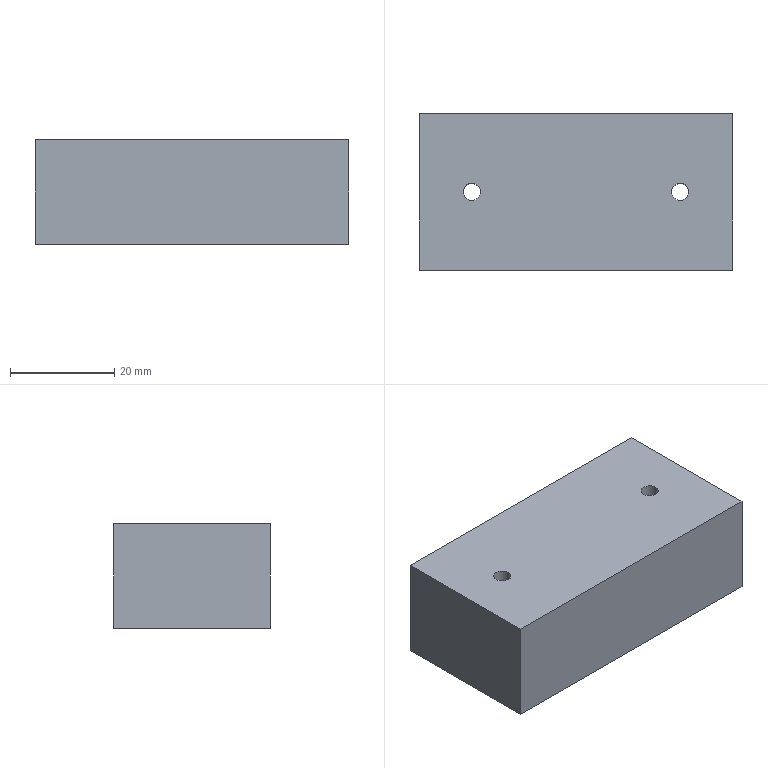Part | NX | features BREP 1 | 1 solid | 10 faces | box 60 x 30 x 20 mm | volume 35658 mm3 | plane 6 | cylinder 4 | commonest cylinder face diameters 3.3 x4
STEP:
#1=CARTESIAN_POINT('',(-21.65,0.,0.));
#2=VERTEX_POINT('',#1);
#3=CARTESIAN_POINT('',(-18.35,0.,0.));
#4=VERTEX_POINT('',#3);
#5=CARTESIAN_POINT('',(-20.,0.,0.));
#6=DIRECTION('',(0.,0.,1.));
#7=DIRECTION('',(1.,0.,0.));
#8=AXIS2_PLACEMENT_3D('',#5,#6,#7);
#9=CIRCLE('',#8,1.65);
#10=EDGE_CURVE('',#2,#4,#9,.T.);
#11=ORIENTED_EDGE('',*,*,#10,.F.);
#12=CARTESIAN_POINT('',(-21.65,0.,20.));
#13=VERTEX_POINT('',#12);
#14=CARTESIAN_POINT('',(-21.65,0.,20.));
#15=DIRECTION('',(0.,0.,1.));
#16=VECTOR('',#15,1000.);
#17=LINE('',#14,#16);
#18=EDGE_CURVE('',#13,#2,#17,.F.);
#19=ORIENTED_EDGE('',*,*,#18,.F.);
#20=CARTESIAN_POINT('',(-18.35,0.,20.));
#21=VERTEX_POINT('',#20);
#22=CARTESIAN_POINT('',(-20.,0.,20.));
#23=DIRECTION('',(0.,0.,1.));
#24=DIRECTION('',(1.,0.,0.));
#25=AXIS2_PLACEMENT_3D('',#22,#23,#24);
#26=CIRCLE('',#25,1.65);
#27=EDGE_CURVE('',#13,#21,#26,.T.);
#28=ORIENTED_EDGE('',*,*,#27,.T.);
#29=CARTESIAN_POINT('',(-18.35,0.,20.));
#30=DIRECTION('',(0.,0.,1.));
#31=VECTOR('',#30,1000.);
#32=LINE('',#29,#31);
#33=EDGE_CURVE('',#21,#4,#32,.F.);
#34=ORIENTED_EDGE('',*,*,#33,.T.);
#35=EDGE_LOOP('',(#11,#19,#28,#34));
#36=FACE_BOUND('',#35,.T.);
#37=CARTESIAN_POINT('',(-20.,0.,20.));
#38=DIRECTION('',(0.,0.,1.));
#39=DIRECTION('',(1.,0.,0.));
#40=AXIS2_PLACEMENT_3D('',#37,#38,#39);
#41=CYLINDRICAL_SURFACE('',#40,1.65);
#42=ADVANCED_FACE('',(#36),#41,.F.);
#43=CARTESIAN_POINT('',(18.35,0.,0.));
#44=VERTEX_POINT('',#43);
#45=CARTESIAN_POINT('',(21.65,0.,0.));
#46=VERTEX_POINT('',#45);
#47=CARTESIAN_POINT('',(20.,0.,0.));
#48=DIRECTION('',(0.,0.,1.));
#49=DIRECTION('',(1.,0.,0.));
#50=AXIS2_PLACEMENT_3D('',#47,#48,#49);
#51=CIRCLE('',#50,1.65);
#52=EDGE_CURVE('',#44,#46,#51,.T.);
#53=ORIENTED_EDGE('',*,*,#52,.F.);
#54=CARTESIAN_POINT('',(18.35,0.,20.));
#55=VERTEX_POINT('',#54);
#56=CARTESIAN_POINT('',(18.35,0.,20.));
#57=DIRECTION('',(0.,0.,1.));
#58=VECTOR('',#57,1000.);
#59=LINE('',#56,#58);
#60=EDGE_CURVE('',#55,#44,#59,.F.);
#61=ORIENTED_EDGE('',*,*,#60,.F.);
#62=CARTESIAN_POINT('',(21.65,0.,20.));
#63=VERTEX_POINT('',#62);
#64=CARTESIAN_POINT('',(20.,0.,20.));
#65=DIRECTION('',(0.,0.,1.));
#66=DIRECTION('',(1.,0.,0.));
#67=AXIS2_PLACEMENT_3D('',#64,#65,#66);
#68=CIRCLE('',#67,1.65);
#69=EDGE_CURVE('',#55,#63,#68,.T.);
#70=ORIENTED_EDGE('',*,*,#69,.T.);
#71=CARTESIAN_POINT('',(21.65,0.,20.));
#72=DIRECTION('',(0.,0.,1.));
#73=VECTOR('',#72,1000.);
#74=LINE('',#71,#73);
#75=EDGE_CURVE('',#63,#46,#74,.F.);
#76=ORIENTED_EDGE('',*,*,#75,.T.);
#77=EDGE_LOOP('',(#53,#61,#70,#76));
#78=FACE_BOUND('',#77,.T.);
#79=CARTESIAN_POINT('',(20.,0.,20.));
#80=DIRECTION('',(0.,0.,1.));
#81=DIRECTION('',(1.,0.,0.));
#82=AXIS2_PLACEMENT_3D('',#79,#80,#81);
#83=CYLINDRICAL_SURFACE('',#82,1.65);
#84=ADVANCED_FACE('',(#78),#83,.F.);
#85=CARTESIAN_POINT('',(30.,-15.,0.));
#86=VERTEX_POINT('',#85);
#87=CARTESIAN_POINT('',(30.,15.,0.));
#88=VERTEX_POINT('',#87);
#89=CARTESIAN_POINT('',(30.,-15.,0.));
#90=DIRECTION('',(0.,1.,0.));
#91=VECTOR('',#90,1000.);
#92=LINE('',#89,#91);
#93=EDGE_CURVE('',#86,#88,#92,.T.);
#94=ORIENTED_EDGE('',*,*,#93,.T.);
#95=CARTESIAN_POINT('',(30.,15.,20.));
#96=VERTEX_POINT('',#95);
#97=CARTESIAN_POINT('',(30.,15.,20.));
#98=DIRECTION('',(0.,0.,-1.));
#99=VECTOR('',#98,1000.);
#100=LINE('',#97,#99);
#101=EDGE_CURVE('',#96,#88,#100,.T.);
#102=ORIENTED_EDGE('',*,*,#101,.F.);
#103=CARTESIAN_POINT('',(30.,-15.,20.));
#104=VERTEX_POINT('',#103);
#105=CARTESIAN_POINT('',(30.,-15.,20.));
#106=DIRECTION('',(0.,1.,0.));
#107=VECTOR('',#106,1000.);
#108=LINE('',#105,#107);
#109=EDGE_CURVE('',#104,#96,#108,.T.);
#110=ORIENTED_EDGE('',*,*,#109,.F.);
#111=CARTESIAN_POINT('',(30.,-15.,20.));
#112=DIRECTION('',(0.,0.,-1.));
#113=VECTOR('',#112,1000.);
#114=LINE('',#111,#113);
#115=EDGE_CURVE('',#104,#86,#114,.T.);
#116=ORIENTED_EDGE('',*,*,#115,.T.);
#117=EDGE_LOOP('',(#94,#102,#110,#116));
#118=FACE_BOUND('',#117,.T.);
#119=CARTESIAN_POINT('',(30.,-15.,20.));
#120=DIRECTION('',(-1.,0.,0.));
#121=DIRECTION('',(0.,0.,1.));
#122=AXIS2_PLACEMENT_3D('',#119,#120,#121);
#123=PLANE('',#122);
#124=ADVANCED_FACE('',(#118),#123,.F.);
#125=CARTESIAN_POINT('',(-30.,15.,0.));
#126=VERTEX_POINT('',#125);
#127=CARTESIAN_POINT('',(-30.,15.,0.));
#128=DIRECTION('',(-1.,0.,0.));
#129=VECTOR('',#128,1000.);
#130=LINE('',#127,#129);
#131=EDGE_CURVE('',#88,#126,#130,.T.);
#132=ORIENTED_EDGE('',*,*,#131,.T.);
#133=CARTESIAN_POINT('',(-30.,15.,20.));
#134=VERTEX_POINT('',#133);
#135=CARTESIAN_POINT('',(-30.,15.,20.));
#136=DIRECTION('',(0.,0.,-1.));
#137=VECTOR('',#136,1000.);
#138=LINE('',#135,#137);
#139=EDGE_CURVE('',#134,#126,#138,.T.);
#140=ORIENTED_EDGE('',*,*,#139,.F.);
#141=CARTESIAN_POINT('',(-30.,15.,20.));
#142=DIRECTION('',(-1.,0.,0.));
#143=VECTOR('',#142,1000.);
#144=LINE('',#141,#143);
#145=EDGE_CURVE('',#96,#134,#144,.T.);
#146=ORIENTED_EDGE('',*,*,#145,.F.);
#147=ORIENTED_EDGE('',*,*,#101,.T.);
#148=EDGE_LOOP('',(#132,#140,#146,#147));
#149=FACE_BOUND('',#148,.T.);
#150=CARTESIAN_POINT('',(-30.,15.,20.));
#151=DIRECTION('',(0.,-1.,0.));
#152=DIRECTION('',(0.,0.,-1.));
#153=AXIS2_PLACEMENT_3D('',#150,#151,#152);
#154=PLANE('',#153);
#155=ADVANCED_FACE('',(#149),#154,.F.);
#156=CARTESIAN_POINT('',(-30.,-15.,0.));
#157=VERTEX_POINT('',#156);
#158=CARTESIAN_POINT('',(-30.,-15.,0.));
#159=DIRECTION('',(0.,-1.,0.));
#160=VECTOR('',#159,1000.);
#161=LINE('',#158,#160);
#162=EDGE_CURVE('',#126,#157,#161,.T.);
#163=ORIENTED_EDGE('',*,*,#162,.T.);
#164=CARTESIAN_POINT('',(-30.,-15.,20.));
#165=VERTEX_POINT('',#164);
#166=CARTESIAN_POINT('',(-30.,-15.,20.));
#167=DIRECTION('',(0.,0.,-1.));
#168=VECTOR('',#167,1000.);
#169=LINE('',#166,#168);
#170=EDGE_CURVE('',#165,#157,#169,.T.);
#171=ORIENTED_EDGE('',*,*,#170,.F.);
#172=CARTESIAN_POINT('',(-30.,-15.,20.));
#173=DIRECTION('',(0.,-1.,0.));
#174=VECTOR('',#173,1000.);
#175=LINE('',#172,#174);
#176=EDGE_CURVE('',#134,#165,#175,.T.);
#177=ORIENTED_EDGE('',*,*,#176,.F.);
#178=ORIENTED_EDGE('',*,*,#139,.T.);
#179=EDGE_LOOP('',(#163,#171,#177,#178));
#180=FACE_BOUND('',#179,.T.);
#181=CARTESIAN_POINT('',(-30.,-15.,20.));
#182=DIRECTION('',(1.,0.,0.));
#183=DIRECTION('',(0.,1.,0.));
#184=AXIS2_PLACEMENT_3D('',#181,#182,#183);
#185=PLANE('',#184);
#186=ADVANCED_FACE('',(#180),#185,.F.);
#187=CARTESIAN_POINT('',(-30.,-15.,0.));
#188=DIRECTION('',(1.,0.,0.));
#189=VECTOR('',#188,1000.);
#190=LINE('',#187,#189);
#191=EDGE_CURVE('',#157,#86,#190,.T.);
#192=ORIENTED_EDGE('',*,*,#191,.T.);
#193=ORIENTED_EDGE('',*,*,#115,.F.);
#194=CARTESIAN_POINT('',(-30.,-15.,20.));
#195=DIRECTION('',(1.,0.,0.));
#196=VECTOR('',#195,1000.);
#197=LINE('',#194,#196);
#198=EDGE_CURVE('',#165,#104,#197,.T.);
#199=ORIENTED_EDGE('',*,*,#198,.F.);
#200=ORIENTED_EDGE('',*,*,#170,.T.);
#201=EDGE_LOOP('',(#192,#193,#199,#200));
#202=FACE_BOUND('',#201,.T.);
#203=CARTESIAN_POINT('',(-30.,-15.,20.));
#204=DIRECTION('',(0.,1.,0.));
#205=DIRECTION('',(1.,0.,0.));
#206=AXIS2_PLACEMENT_3D('',#203,#204,#205);
#207=PLANE('',#206);
#208=ADVANCED_FACE('',(#202),#207,.F.);
#209=ORIENTED_EDGE('',*,*,#109,.T.);
#210=ORIENTED_EDGE('',*,*,#145,.T.);
#211=ORIENTED_EDGE('',*,*,#176,.T.);
#212=ORIENTED_EDGE('',*,*,#198,.T.);
#213=EDGE_LOOP('',(#209,#210,#211,#212));
#214=FACE_BOUND('',#213,.T.);
#215=CARTESIAN_POINT('',(-20.,0.,20.));
#216=DIRECTION('',(0.,0.,1.));
#217=DIRECTION('',(1.,0.,0.));
#218=AXIS2_PLACEMENT_3D('',#215,#216,#217);
#219=CIRCLE('',#218,1.65);
#220=EDGE_CURVE('',#21,#13,#219,.T.);
#221=ORIENTED_EDGE('',*,*,#220,.F.);
#222=ORIENTED_EDGE('',*,*,#27,.F.);
#223=EDGE_LOOP('',(#221,#222));
#224=FACE_BOUND('',#223,.T.);
#225=CARTESIAN_POINT('',(20.,0.,20.));
#226=DIRECTION('',(0.,0.,1.));
#227=DIRECTION('',(1.,0.,0.));
#228=AXIS2_PLACEMENT_3D('',#225,#226,#227);
#229=CIRCLE('',#228,1.65);
#230=EDGE_CURVE('',#63,#55,#229,.T.);
#231=ORIENTED_EDGE('',*,*,#230,.F.);
#232=ORIENTED_EDGE('',*,*,#69,.F.);
#233=EDGE_LOOP('',(#231,#232));
#234=FACE_BOUND('',#233,.T.);
#235=CARTESIAN_POINT('',(0.,0.,20.));
#236=DIRECTION('',(0.,0.,-1.));
#237=DIRECTION('',(0.,-1.,0.));
#238=AXIS2_PLACEMENT_3D('',#235,#236,#237);
#239=PLANE('',#238);
#240=ADVANCED_FACE('',(#214,#224,#234),#239,.F.);
#241=ORIENTED_EDGE('',*,*,#93,.F.);
#242=ORIENTED_EDGE('',*,*,#191,.F.);
#243=ORIENTED_EDGE('',*,*,#162,.F.);
#244=ORIENTED_EDGE('',*,*,#131,.F.);
#245=EDGE_LOOP('',(#241,#242,#243,#244));
#246=FACE_BOUND('',#245,.T.);
#247=CARTESIAN_POINT('',(-20.,0.,0.));
#248=DIRECTION('',(0.,0.,1.));
#249=DIRECTION('',(1.,0.,0.));
#250=AXIS2_PLACEMENT_3D('',#247,#248,#249);
#251=CIRCLE('',#250,1.65);
#252=EDGE_CURVE('',#4,#2,#251,.T.);
#253=ORIENTED_EDGE('',*,*,#252,.T.);
#254=ORIENTED_EDGE('',*,*,#10,.T.);
#255=EDGE_LOOP('',(#253,#254));
#256=FACE_BOUND('',#255,.T.);
#257=CARTESIAN_POINT('',(20.,0.,0.));
#258=DIRECTION('',(0.,0.,1.));
#259=DIRECTION('',(1.,0.,0.));
#260=AXIS2_PLACEMENT_3D('',#257,#258,#259);
#261=CIRCLE('',#260,1.65);
#262=EDGE_CURVE('',#46,#44,#261,.T.);
#263=ORIENTED_EDGE('',*,*,#262,.T.);
#264=ORIENTED_EDGE('',*,*,#52,.T.);
#265=EDGE_LOOP('',(#263,#264));
#266=FACE_BOUND('',#265,.T.);
#267=CARTESIAN_POINT('',(0.,0.,0.));
#268=DIRECTION('',(0.,0.,-1.));
#269=DIRECTION('',(0.,-1.,0.));
#270=AXIS2_PLACEMENT_3D('',#267,#268,#269);
#271=PLANE('',#270);
#272=ADVANCED_FACE('',(#246,#256,#266),#271,.T.);
#273=ORIENTED_EDGE('',*,*,#60,.T.);
#274=ORIENTED_EDGE('',*,*,#262,.F.);
#275=ORIENTED_EDGE('',*,*,#75,.F.);
#276=ORIENTED_EDGE('',*,*,#230,.T.);
#277=EDGE_LOOP('',(#273,#274,#275,#276));
#278=FACE_BOUND('',#277,.T.);
#279=CARTESIAN_POINT('',(20.,0.,20.));
#280=DIRECTION('',(0.,0.,1.));
#281=DIRECTION('',(1.,0.,0.));
#282=AXIS2_PLACEMENT_3D('',#279,#280,#281);
#283=CYLINDRICAL_SURFACE('',#282,1.65);
#284=ADVANCED_FACE('',(#278),#283,.F.);
#285=ORIENTED_EDGE('',*,*,#18,.T.);
#286=ORIENTED_EDGE('',*,*,#252,.F.);
#287=ORIENTED_EDGE('',*,*,#33,.F.);
#288=ORIENTED_EDGE('',*,*,#220,.T.);
#289=EDGE_LOOP('',(#285,#286,#287,#288));
#290=FACE_BOUND('',#289,.T.);
#291=CARTESIAN_POINT('',(-20.,0.,20.));
#292=DIRECTION('',(0.,0.,1.));
#293=DIRECTION('',(1.,0.,0.));
#294=AXIS2_PLACEMENT_3D('',#291,#292,#293);
#295=CYLINDRICAL_SURFACE('',#294,1.65);
#296=ADVANCED_FACE('',(#290),#295,.F.);
#297=CLOSED_SHELL('',(#42,#84,#124,#155,#186,#208,#240,#272,#284,#296));
#298=MANIFOLD_SOLID_BREP('',#297);
#299=(LENGTH_UNIT()NAMED_UNIT(*)SI_UNIT(.MILLI.,.METRE.));
#300=UNCERTAINTY_MEASURE_WITH_UNIT(LENGTH_MEASURE(0.00001),#299,'','');
#301=(NAMED_UNIT(*)PLANE_ANGLE_UNIT()SI_UNIT($,.RADIAN.));
#302=(NAMED_UNIT(*)SI_UNIT($,.STERADIAN.)SOLID_ANGLE_UNIT());
#303=(GEOMETRIC_REPRESENTATION_CONTEXT(3)GLOBAL_UNCERTAINTY_ASSIGNED_CONTEXT((#300))GLOBAL_UNIT_ASSIGNED_CONTEXT((#299,#301,#302))REPRESENTATION_CONTEXT('',''));
#304=ADVANCED_BREP_SHAPE_REPRESENTATION('',(#298),#303);